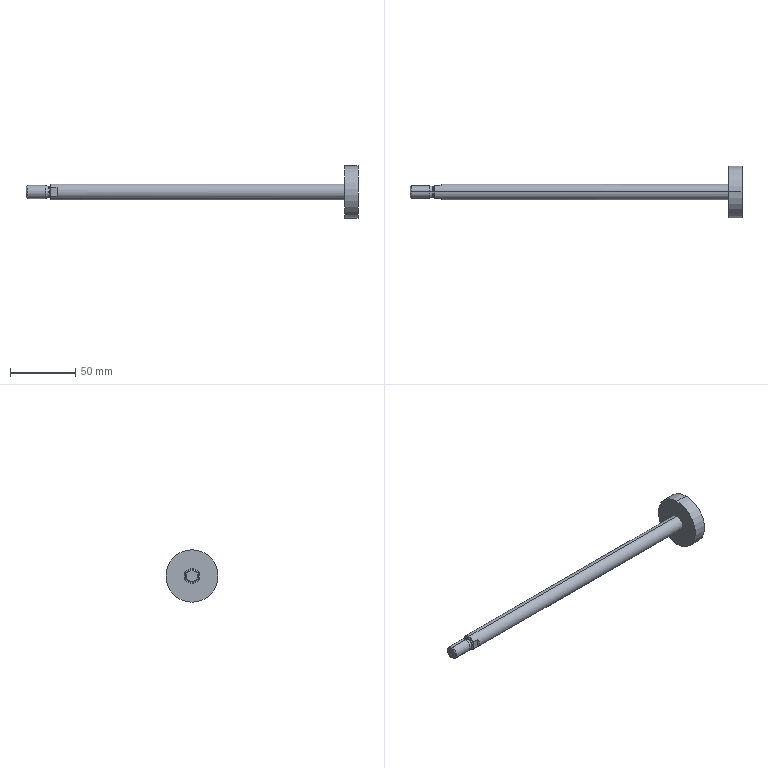Part | SolidWorks | features ICE 6, Draft 2, Chamfer 1, Fillet 1, Revolution 1 | 1 solid | 24 faces | box 253.7 x 40 x 40 mm | volume 39349 mm3 | cylinder 8 | plane 8 | torus 4 | cone 4 | commonest cylinder face diameters 8.2 x2 10 x2 12 x2 40 x2
STEP:
#1=CARTESIAN_POINT('',(-7.699,0.,-4.136));
#2=VERTEX_POINT('',#1);
#3=CARTESIAN_POINT('',(-7.699,0.,4.136));
#4=VERTEX_POINT('',#3);
#5=CARTESIAN_POINT('',(-7.699,0.,0.));
#6=DIRECTION('',(-1.,0.,0.));
#7=DIRECTION('',(0.,0.,1.));
#8=AXIS2_PLACEMENT_3D('',#5,#6,#7);
#9=CIRCLE('',#8,4.136);
#10=EDGE_CURVE('',#2,#4,#9,.T.);
#11=ORIENTED_EDGE('',*,*,#10,.F.);
#12=CARTESIAN_POINT('',(-7.494,0.,-4.1));
#13=VERTEX_POINT('',#12);
#14=CARTESIAN_POINT('',(-7.494,0.,-4.7));
#15=DIRECTION('',(0.,1.,0.));
#16=DIRECTION('',(0.,0.,1.));
#17=AXIS2_PLACEMENT_3D('',#14,#15,#16);
#18=CIRCLE('',#17,0.6);
#19=EDGE_CURVE('',#2,#13,#18,.T.);
#20=ORIENTED_EDGE('',*,*,#19,.T.);
#21=CARTESIAN_POINT('',(-7.494,0.,4.1));
#22=VERTEX_POINT('',#21);
#23=CARTESIAN_POINT('',(-7.494,0.,0.));
#24=DIRECTION('',(1.,0.,0.));
#25=DIRECTION('',(0.,0.,1.));
#26=AXIS2_PLACEMENT_3D('',#23,#24,#25);
#27=CIRCLE('',#26,4.1);
#28=EDGE_CURVE('',#22,#13,#27,.T.);
#29=ORIENTED_EDGE('',*,*,#28,.F.);
#30=CARTESIAN_POINT('',(-7.494,0.,4.7));
#31=DIRECTION('',(0.,-1.,0.));
#32=DIRECTION('',(0.,0.,-1.));
#33=AXIS2_PLACEMENT_3D('',#30,#31,#32);
#34=CIRCLE('',#33,0.6);
#35=EDGE_CURVE('',#4,#22,#34,.T.);
#36=ORIENTED_EDGE('',*,*,#35,.F.);
#37=EDGE_LOOP('',(#11,#20,#29,#36));
#38=FACE_OUTER_BOUND('',#37,.T.);
#39=CARTESIAN_POINT('',(-7.494,0.,0.));
#40=DIRECTION('',(-1.,0.,0.));
#41=DIRECTION('',(0.,0.,1.));
#42=AXIS2_PLACEMENT_3D('',#39,#40,#41);
#43=TOROIDAL_SURFACE('',#42,4.7,0.6);
#44=ADVANCED_FACE('',(#38),#43,.F.);
#45=CARTESIAN_POINT('',(-6.7,0.,-4.1));
#46=VERTEX_POINT('',#45);
#47=CARTESIAN_POINT('',(-6.7,0.,4.1));
#48=VERTEX_POINT('',#47);
#49=CARTESIAN_POINT('',(-6.7,0.,0.));
#50=DIRECTION('',(-1.,0.,0.));
#51=DIRECTION('',(0.,0.,1.));
#52=AXIS2_PLACEMENT_3D('',#49,#50,#51);
#53=CIRCLE('',#52,4.1);
#54=EDGE_CURVE('',#46,#48,#53,.T.);
#55=ORIENTED_EDGE('',*,*,#54,.F.);
#56=CARTESIAN_POINT('',(-6.1,0.,-4.7));
#57=VERTEX_POINT('',#56);
#58=CARTESIAN_POINT('',(-6.7,0.,-4.7));
#59=DIRECTION('',(0.,1.,0.));
#60=DIRECTION('',(0.,0.,1.));
#61=AXIS2_PLACEMENT_3D('',#58,#59,#60);
#62=CIRCLE('',#61,0.6);
#63=EDGE_CURVE('',#46,#57,#62,.T.);
#64=ORIENTED_EDGE('',*,*,#63,.T.);
#65=CARTESIAN_POINT('',(-6.1,0.,4.7));
#66=VERTEX_POINT('',#65);
#67=CARTESIAN_POINT('',(-6.1,0.,0.));
#68=DIRECTION('',(1.,0.,0.));
#69=DIRECTION('',(0.,0.,1.));
#70=AXIS2_PLACEMENT_3D('',#67,#68,#69);
#71=CIRCLE('',#70,4.7);
#72=EDGE_CURVE('',#66,#57,#71,.T.);
#73=ORIENTED_EDGE('',*,*,#72,.F.);
#74=CARTESIAN_POINT('',(-6.7,0.,4.7));
#75=DIRECTION('',(0.,-1.,0.));
#76=DIRECTION('',(0.,0.,-1.));
#77=AXIS2_PLACEMENT_3D('',#74,#75,#76);
#78=CIRCLE('',#77,0.6);
#79=EDGE_CURVE('',#48,#66,#78,.T.);
#80=ORIENTED_EDGE('',*,*,#79,.F.);
#81=EDGE_LOOP('',(#55,#64,#73,#80));
#82=FACE_OUTER_BOUND('',#81,.T.);
#83=CARTESIAN_POINT('',(-6.7,0.,0.));
#84=DIRECTION('',(-1.,0.,0.));
#85=DIRECTION('',(0.,0.,1.));
#86=AXIS2_PLACEMENT_3D('',#83,#84,#85);
#87=TOROIDAL_SURFACE('',#86,4.7,0.6);
#88=ADVANCED_FACE('',(#82),#87,.F.);
#89=CARTESIAN_POINT('',(-25.1,0.,4.233));
#90=VERTEX_POINT('',#89);
#91=CARTESIAN_POINT('',(-25.1,0.,-4.233));
#92=VERTEX_POINT('',#91);
#93=CARTESIAN_POINT('',(-25.1,0.,0.));
#94=DIRECTION('',(-1.,0.,0.));
#95=DIRECTION('',(0.,0.,1.));
#96=AXIS2_PLACEMENT_3D('',#93,#94,#95);
#97=CIRCLE('',#96,4.233);
#98=EDGE_CURVE('',#90,#92,#97,.T.);
#99=ORIENTED_EDGE('',*,*,#98,.F.);
#100=CARTESIAN_POINT('',(-24.333,0.,5.));
#101=VERTEX_POINT('',#100);
#102=CARTESIAN_POINT('',(-25.1,0.,4.233));
#103=DIRECTION('',(0.7071,0.,0.7071));
#104=VECTOR('',#103,1000.);
#105=LINE('',#102,#104);
#106=EDGE_CURVE('',#90,#101,#105,.T.);
#107=ORIENTED_EDGE('',*,*,#106,.T.);
#108=CARTESIAN_POINT('',(-24.333,0.,-5.));
#109=VERTEX_POINT('',#108);
#110=CARTESIAN_POINT('',(-24.333,0.,0.));
#111=DIRECTION('',(1.,0.,0.));
#112=DIRECTION('',(0.,0.,1.));
#113=AXIS2_PLACEMENT_3D('',#110,#111,#112);
#114=CIRCLE('',#113,5.);
#115=EDGE_CURVE('',#109,#101,#114,.T.);
#116=ORIENTED_EDGE('',*,*,#115,.F.);
#117=CARTESIAN_POINT('',(-25.1,0.,-4.233));
#118=DIRECTION('',(0.7071,0.,-0.7071));
#119=VECTOR('',#118,1000.);
#120=LINE('',#117,#119);
#121=EDGE_CURVE('',#92,#109,#120,.T.);
#122=ORIENTED_EDGE('',*,*,#121,.F.);
#123=EDGE_LOOP('',(#99,#107,#116,#122));
#124=FACE_OUTER_BOUND('',#123,.T.);
#125=CARTESIAN_POINT('',(-25.1,0.,0.));
#126=DIRECTION('',(1.,0.,0.));
#127=DIRECTION('',(0.,0.,-1.));
#128=AXIS2_PLACEMENT_3D('',#125,#126,#127);
#129=CONICAL_SURFACE('',#128,4.233,0.7854);
#130=ADVANCED_FACE('',(#124),#129,.T.);
#131=ORIENTED_EDGE('',*,*,#115,.T.);
#132=CARTESIAN_POINT('',(-10.073,0.,5.));
#133=VERTEX_POINT('',#132);
#134=CARTESIAN_POINT('',(-25.1,0.,5.));
#135=DIRECTION('',(1.,0.,0.));
#136=VECTOR('',#135,1000.);
#137=LINE('',#134,#136);
#138=EDGE_CURVE('',#101,#133,#137,.T.);
#139=ORIENTED_EDGE('',*,*,#138,.T.);
#140=CARTESIAN_POINT('',(-10.073,0.,-5.));
#141=VERTEX_POINT('',#140);
#142=CARTESIAN_POINT('',(-10.073,0.,0.));
#143=DIRECTION('',(-1.,0.,0.));
#144=DIRECTION('',(0.,0.,1.));
#145=AXIS2_PLACEMENT_3D('',#142,#143,#144);
#146=CIRCLE('',#145,5.);
#147=EDGE_CURVE('',#133,#141,#146,.T.);
#148=ORIENTED_EDGE('',*,*,#147,.T.);
#149=CARTESIAN_POINT('',(-25.1,0.,-5.));
#150=DIRECTION('',(1.,0.,0.));
#151=VECTOR('',#150,1000.);
#152=LINE('',#149,#151);
#153=EDGE_CURVE('',#109,#141,#152,.T.);
#154=ORIENTED_EDGE('',*,*,#153,.F.);
#155=EDGE_LOOP('',(#131,#139,#148,#154));
#156=FACE_OUTER_BOUND('',#155,.T.);
#157=CARTESIAN_POINT('',(-25.1,0.,0.));
#158=DIRECTION('',(1.,0.,0.));
#159=DIRECTION('',(0.,0.,-1.));
#160=AXIS2_PLACEMENT_3D('',#157,#158,#159);
#161=CYLINDRICAL_SURFACE('',#160,5.);
#162=ADVANCED_FACE('',(#156),#161,.T.);
#163=CARTESIAN_POINT('',(-7.699,0.,0.));
#164=DIRECTION('',(-1.,0.,0.));
#165=DIRECTION('',(0.,0.,1.));
#166=AXIS2_PLACEMENT_3D('',#163,#164,#165);
#167=CIRCLE('',#166,4.136);
#168=EDGE_CURVE('',#4,#2,#167,.T.);
#169=ORIENTED_EDGE('',*,*,#168,.T.);
#170=CARTESIAN_POINT('',(-7.6,0.,-4.1));
#171=DIRECTION('',(-0.9397,0.,-0.342));
#172=VECTOR('',#171,1000.);
#173=LINE('',#170,#172);
#174=EDGE_CURVE('',#2,#141,#173,.T.);
#175=ORIENTED_EDGE('',*,*,#174,.T.);
#176=ORIENTED_EDGE('',*,*,#147,.F.);
#177=CARTESIAN_POINT('',(-7.6,0.,4.1));
#178=DIRECTION('',(-0.9397,0.,0.342));
#179=VECTOR('',#178,1000.);
#180=LINE('',#177,#179);
#181=EDGE_CURVE('',#4,#133,#180,.T.);
#182=ORIENTED_EDGE('',*,*,#181,.F.);
#183=EDGE_LOOP('',(#169,#175,#176,#182));
#184=FACE_OUTER_BOUND('',#183,.T.);
#185=CARTESIAN_POINT('',(-7.6,0.,0.));
#186=DIRECTION('',(-1.,0.,0.));
#187=DIRECTION('',(0.,0.,1.));
#188=AXIS2_PLACEMENT_3D('',#185,#186,#187);
#189=CONICAL_SURFACE('',#188,4.1,0.3491);
#190=ADVANCED_FACE('',(#184),#189,.T.);
#191=CARTESIAN_POINT('',(-7.494,0.,0.));
#192=DIRECTION('',(1.,0.,0.));
#193=DIRECTION('',(0.,0.,1.));
#194=AXIS2_PLACEMENT_3D('',#191,#192,#193);
#195=CIRCLE('',#194,4.1);
#196=EDGE_CURVE('',#13,#22,#195,.T.);
#197=ORIENTED_EDGE('',*,*,#196,.T.);
#198=CARTESIAN_POINT('',(-7.6,0.,4.1));
#199=DIRECTION('',(1.,0.,0.));
#200=VECTOR('',#199,1000.);
#201=LINE('',#198,#200);
#202=EDGE_CURVE('',#22,#48,#201,.T.);
#203=ORIENTED_EDGE('',*,*,#202,.T.);
#204=CARTESIAN_POINT('',(-6.7,0.,0.));
#205=DIRECTION('',(-1.,0.,0.));
#206=DIRECTION('',(0.,0.,1.));
#207=AXIS2_PLACEMENT_3D('',#204,#205,#206);
#208=CIRCLE('',#207,4.1);
#209=EDGE_CURVE('',#48,#46,#208,.T.);
#210=ORIENTED_EDGE('',*,*,#209,.T.);
#211=CARTESIAN_POINT('',(-7.6,0.,-4.1));
#212=DIRECTION('',(1.,0.,0.));
#213=VECTOR('',#212,1000.);
#214=LINE('',#211,#213);
#215=EDGE_CURVE('',#13,#46,#214,.T.);
#216=ORIENTED_EDGE('',*,*,#215,.F.);
#217=EDGE_LOOP('',(#197,#203,#210,#216));
#218=FACE_OUTER_BOUND('',#217,.T.);
#219=CARTESIAN_POINT('',(-7.6,0.,0.));
#220=DIRECTION('',(1.,0.,0.));
#221=DIRECTION('',(0.,0.,-1.));
#222=AXIS2_PLACEMENT_3D('',#219,#220,#221);
#223=CYLINDRICAL_SURFACE('',#222,4.1);
#224=ADVANCED_FACE('',(#218),#223,.T.);
#225=CARTESIAN_POINT('',(-6.1,0.,6.));
#226=VERTEX_POINT('',#225);
#227=CARTESIAN_POINT('',(-6.1,5.,3.317));
#228=VERTEX_POINT('',#227);
#229=CARTESIAN_POINT('',(-6.1,0.,0.));
#230=DIRECTION('',(-1.,0.,0.));
#231=DIRECTION('',(0.,0.,1.));
#232=AXIS2_PLACEMENT_3D('',#229,#230,#231);
#233=CIRCLE('',#232,6.);
#234=EDGE_CURVE('',#226,#228,#233,.T.);
#235=ORIENTED_EDGE('',*,*,#234,.F.);
#236=CARTESIAN_POINT('',(218.6,0.,6.));
#237=VERTEX_POINT('',#236);
#238=CARTESIAN_POINT('',(-6.1,0.,6.));
#239=DIRECTION('',(1.,0.,0.));
#240=VECTOR('',#239,1000.);
#241=LINE('',#238,#240);
#242=EDGE_CURVE('',#226,#237,#241,.T.);
#243=ORIENTED_EDGE('',*,*,#242,.T.);
#244=CARTESIAN_POINT('',(218.6,0.,-6.));
#245=VERTEX_POINT('',#244);
#246=CARTESIAN_POINT('',(218.6,0.,0.));
#247=DIRECTION('',(-1.,0.,0.));
#248=DIRECTION('',(0.,0.,1.));
#249=AXIS2_PLACEMENT_3D('',#246,#247,#248);
#250=CIRCLE('',#249,6.);
#251=EDGE_CURVE('',#237,#245,#250,.T.);
#252=ORIENTED_EDGE('',*,*,#251,.T.);
#253=CARTESIAN_POINT('',(-6.1,0.,-6.));
#254=VERTEX_POINT('',#253);
#255=CARTESIAN_POINT('',(-6.1,0.,-6.));
#256=DIRECTION('',(1.,0.,0.));
#257=VECTOR('',#256,1000.);
#258=LINE('',#255,#257);
#259=EDGE_CURVE('',#254,#245,#258,.T.);
#260=ORIENTED_EDGE('',*,*,#259,.F.);
#261=CARTESIAN_POINT('',(-6.1,5.,-3.317));
#262=VERTEX_POINT('',#261);
#263=CARTESIAN_POINT('',(-6.1,0.,0.));
#264=DIRECTION('',(-1.,0.,0.));
#265=DIRECTION('',(0.,0.,1.));
#266=AXIS2_PLACEMENT_3D('',#263,#264,#265);
#267=CIRCLE('',#266,6.);
#268=EDGE_CURVE('',#262,#254,#267,.T.);
#269=ORIENTED_EDGE('',*,*,#268,.F.);
#270=CARTESIAN_POINT('',(-1.4,5.,-3.317));
#271=VERTEX_POINT('',#270);
#272=CARTESIAN_POINT('',(-1.4,5.,-3.317));
#273=DIRECTION('',(-1.,0.,0.));
#274=VECTOR('',#273,1000.);
#275=LINE('',#272,#274);
#276=EDGE_CURVE('',#271,#262,#275,.T.);
#277=ORIENTED_EDGE('',*,*,#276,.F.);
#278=CARTESIAN_POINT('',(-1.4,5.,3.317));
#279=VERTEX_POINT('',#278);
#280=CARTESIAN_POINT('',(-1.4,5.,3.317));
#281=CARTESIAN_POINT('',(-0.6061,6.375,1.244));
#282=CARTESIAN_POINT('',(-0.6061,6.375,-1.244));
#283=CARTESIAN_POINT('',(-1.4,5.,-3.317));
#284=(BOUNDED_CURVE()B_SPLINE_CURVE(3,(#280,#281,#282,#283),.UNSPECIFIED.,.F.,.F.)B_SPLINE_CURVE_WITH_KNOTS((4,4),(5.697,6.869),.UNSPECIFIED.)CURVE()GEOMETRIC_REPRESENTATION_ITEM()RATIONAL_B_SPLINE_CURVE((1.,0.8889,0.8889,1.))REPRESENTATION_ITEM(''));
#285=EDGE_CURVE('',#279,#271,#284,.T.);
#286=ORIENTED_EDGE('',*,*,#285,.F.);
#287=CARTESIAN_POINT('',(-1.4,5.,3.317));
#288=DIRECTION('',(-1.,0.,0.));
#289=VECTOR('',#288,1000.);
#290=LINE('',#287,#289);
#291=EDGE_CURVE('',#279,#228,#290,.T.);
#292=ORIENTED_EDGE('',*,*,#291,.T.);
#293=EDGE_LOOP('',(#235,#243,#252,#260,#269,#277,#286,#292));
#294=FACE_OUTER_BOUND('',#293,.T.);
#295=CARTESIAN_POINT('',(-6.1,0.,0.));
#296=DIRECTION('',(1.,0.,0.));
#297=DIRECTION('',(0.,0.,-1.));
#298=AXIS2_PLACEMENT_3D('',#295,#296,#297);
#299=CYLINDRICAL_SURFACE('',#298,6.);
#300=ADVANCED_FACE('',(#294),#299,.T.);
#301=CARTESIAN_POINT('',(228.6,0.,20.));
#302=VERTEX_POINT('',#301);
#303=CARTESIAN_POINT('',(228.6,0.,-20.));
#304=VERTEX_POINT('',#303);
#305=CARTESIAN_POINT('',(228.6,0.,0.));
#306=DIRECTION('',(-1.,0.,0.));
#307=DIRECTION('',(0.,0.,1.));
#308=AXIS2_PLACEMENT_3D('',#305,#306,#307);
#309=CIRCLE('',#308,20.);
#310=EDGE_CURVE('',#302,#304,#309,.T.);
#311=ORIENTED_EDGE('',*,*,#310,.T.);
#312=CARTESIAN_POINT('',(218.6,0.,-20.));
#313=VERTEX_POINT('',#312);
#314=CARTESIAN_POINT('',(228.6,0.,-20.));
#315=DIRECTION('',(-1.,0.,0.));
#316=VECTOR('',#315,1000.);
#317=LINE('',#314,#316);
#318=EDGE_CURVE('',#304,#313,#317,.T.);
#319=ORIENTED_EDGE('',*,*,#318,.T.);
#320=CARTESIAN_POINT('',(218.6,0.,20.));
#321=VERTEX_POINT('',#320);
#322=CARTESIAN_POINT('',(218.6,0.,0.));
#323=DIRECTION('',(-1.,0.,0.));
#324=DIRECTION('',(0.,0.,1.));
#325=AXIS2_PLACEMENT_3D('',#322,#323,#324);
#326=CIRCLE('',#325,20.);
#327=EDGE_CURVE('',#321,#313,#326,.T.);
#328=ORIENTED_EDGE('',*,*,#327,.F.);
#329=CARTESIAN_POINT('',(228.6,0.,20.));
#330=DIRECTION('',(-1.,0.,0.));
#331=VECTOR('',#330,1000.);
#332=LINE('',#329,#331);
#333=EDGE_CURVE('',#302,#321,#332,.T.);
#334=ORIENTED_EDGE('',*,*,#333,.F.);
#335=EDGE_LOOP('',(#311,#319,#328,#334));
#336=FACE_OUTER_BOUND('',#335,.T.);
#337=CARTESIAN_POINT('',(228.6,0.,0.));
#338=DIRECTION('',(-1.,0.,0.));
#339=DIRECTION('',(0.,0.,1.));
#340=AXIS2_PLACEMENT_3D('',#337,#338,#339);
#341=CYLINDRICAL_SURFACE('',#340,20.);
#342=ADVANCED_FACE('',(#336),#341,.T.);
#343=ORIENTED_EDGE('',*,*,#318,.F.);
#344=CARTESIAN_POINT('',(228.6,0.,0.));
#345=DIRECTION('',(-1.,0.,0.));
#346=DIRECTION('',(0.,0.,1.));
#347=AXIS2_PLACEMENT_3D('',#344,#345,#346);
#348=CIRCLE('',#347,20.);
#349=EDGE_CURVE('',#304,#302,#348,.T.);
#350=ORIENTED_EDGE('',*,*,#349,.T.);
#351=ORIENTED_EDGE('',*,*,#333,.T.);
#352=CARTESIAN_POINT('',(218.6,0.,0.));
#353=DIRECTION('',(-1.,0.,0.));
#354=DIRECTION('',(0.,0.,1.));
#355=AXIS2_PLACEMENT_3D('',#352,#353,#354);
#356=CIRCLE('',#355,20.);
#357=EDGE_CURVE('',#313,#321,#356,.T.);
#358=ORIENTED_EDGE('',*,*,#357,.F.);
#359=EDGE_LOOP('',(#343,#350,#351,#358));
#360=FACE_OUTER_BOUND('',#359,.T.);
#361=CARTESIAN_POINT('',(228.6,0.,0.));
#362=DIRECTION('',(-1.,0.,0.));
#363=DIRECTION('',(0.,0.,1.));
#364=AXIS2_PLACEMENT_3D('',#361,#362,#363);
#365=CYLINDRICAL_SURFACE('',#364,20.);
#366=ADVANCED_FACE('',(#360),#365,.T.);
#367=ORIENTED_EDGE('',*,*,#310,.F.);
#368=ORIENTED_EDGE('',*,*,#349,.F.);
#369=EDGE_LOOP('',(#367,#368));
#370=FACE_OUTER_BOUND('',#369,.T.);
#371=CARTESIAN_POINT('',(228.6,20.,0.));
#372=DIRECTION('',(1.,0.,0.));
#373=DIRECTION('',(0.,0.,-1.));
#374=AXIS2_PLACEMENT_3D('',#371,#372,#373);
#375=PLANE('',#374);
#376=ADVANCED_FACE('',(#370),#375,.T.);
#377=CARTESIAN_POINT('',(218.6,0.,0.));
#378=DIRECTION('',(-1.,0.,0.));
#379=DIRECTION('',(0.,0.,1.));
#380=AXIS2_PLACEMENT_3D('',#377,#378,#379);
#381=CIRCLE('',#380,6.);
#382=EDGE_CURVE('',#245,#237,#381,.T.);
#383=ORIENTED_EDGE('',*,*,#382,.F.);
#384=ORIENTED_EDGE('',*,*,#251,.F.);
#385=EDGE_LOOP('',(#383,#384));
#386=FACE_BOUND('',#385,.T.);
#387=ORIENTED_EDGE('',*,*,#327,.T.);
#388=ORIENTED_EDGE('',*,*,#357,.T.);
#389=EDGE_LOOP('',(#387,#388));
#390=FACE_OUTER_BOUND('',#389,.T.);
#391=CARTESIAN_POINT('',(218.6,0.,0.));
#392=DIRECTION('',(-1.,0.,0.));
#393=DIRECTION('',(0.,0.,1.));
#394=AXIS2_PLACEMENT_3D('',#391,#392,#393);
#395=PLANE('',#394);
#396=ADVANCED_FACE('',(#386,#390),#395,.T.);
#397=ORIENTED_EDGE('',*,*,#242,.F.);
#398=CARTESIAN_POINT('',(-6.1,-5.,3.317));
#399=VERTEX_POINT('',#398);
#400=CARTESIAN_POINT('',(-6.1,0.,0.));
#401=DIRECTION('',(-1.,0.,0.));
#402=DIRECTION('',(0.,0.,1.));
#403=AXIS2_PLACEMENT_3D('',#400,#401,#402);
#404=CIRCLE('',#403,6.);
#405=EDGE_CURVE('',#399,#226,#404,.T.);
#406=ORIENTED_EDGE('',*,*,#405,.F.);
#407=CARTESIAN_POINT('',(-1.4,-5.,3.317));
#408=VERTEX_POINT('',#407);
#409=CARTESIAN_POINT('',(-1.4,-5.,3.317));
#410=DIRECTION('',(-1.,0.,0.));
#411=VECTOR('',#410,1000.);
#412=LINE('',#409,#411);
#413=EDGE_CURVE('',#408,#399,#412,.T.);
#414=ORIENTED_EDGE('',*,*,#413,.F.);
#415=CARTESIAN_POINT('',(-1.4,-5.,-3.317));
#416=VERTEX_POINT('',#415);
#417=CARTESIAN_POINT('',(-1.4,-5.,-3.317));
#418=CARTESIAN_POINT('',(-0.6061,-6.375,-1.244));
#419=CARTESIAN_POINT('',(-0.6061,-6.375,1.244));
#420=CARTESIAN_POINT('',(-1.4,-5.,3.317));
#421=(BOUNDED_CURVE()B_SPLINE_CURVE(3,(#417,#418,#419,#420),.UNSPECIFIED.,.F.,.F.)B_SPLINE_CURVE_WITH_KNOTS((4,4),(5.697,6.869),.UNSPECIFIED.)CURVE()GEOMETRIC_REPRESENTATION_ITEM()RATIONAL_B_SPLINE_CURVE((1.,0.8889,0.8889,1.))REPRESENTATION_ITEM(''));
#422=EDGE_CURVE('',#416,#408,#421,.T.);
#423=ORIENTED_EDGE('',*,*,#422,.F.);
#424=CARTESIAN_POINT('',(-6.1,-5.,-3.317));
#425=VERTEX_POINT('',#424);
#426=CARTESIAN_POINT('',(-1.4,-5.,-3.317));
#427=DIRECTION('',(-1.,0.,0.));
#428=VECTOR('',#427,1000.);
#429=LINE('',#426,#428);
#430=EDGE_CURVE('',#416,#425,#429,.T.);
#431=ORIENTED_EDGE('',*,*,#430,.T.);
#432=CARTESIAN_POINT('',(-6.1,0.,0.));
#433=DIRECTION('',(-1.,0.,0.));
#434=DIRECTION('',(0.,0.,1.));
#435=AXIS2_PLACEMENT_3D('',#432,#433,#434);
#436=CIRCLE('',#435,6.);
#437=EDGE_CURVE('',#254,#425,#436,.T.);
#438=ORIENTED_EDGE('',*,*,#437,.F.);
#439=ORIENTED_EDGE('',*,*,#259,.T.);
#440=ORIENTED_EDGE('',*,*,#382,.T.);
#441=EDGE_LOOP('',(#397,#406,#414,#423,#431,#438,#439,#440));
#442=FACE_OUTER_BOUND('',#441,.T.);
#443=CARTESIAN_POINT('',(-6.1,0.,0.));
#444=DIRECTION('',(1.,0.,0.));
#445=DIRECTION('',(0.,0.,-1.));
#446=AXIS2_PLACEMENT_3D('',#443,#444,#445);
#447=CYLINDRICAL_SURFACE('',#446,6.);
#448=ADVANCED_FACE('',(#442),#447,.T.);
#449=ORIENTED_EDGE('',*,*,#72,.T.);
#450=CARTESIAN_POINT('',(-6.1,0.,0.));
#451=DIRECTION('',(1.,0.,0.));
#452=DIRECTION('',(0.,0.,1.));
#453=AXIS2_PLACEMENT_3D('',#450,#451,#452);
#454=CIRCLE('',#453,4.7);
#455=EDGE_CURVE('',#57,#66,#454,.T.);
#456=ORIENTED_EDGE('',*,*,#455,.T.);
#457=EDGE_LOOP('',(#449,#456));
#458=FACE_BOUND('',#457,.T.);
#459=CARTESIAN_POINT('',(-6.1,-5.,3.317));
#460=DIRECTION('',(0.,0.,-1.));
#461=VECTOR('',#460,1000.);
#462=LINE('',#459,#461);
#463=EDGE_CURVE('',#399,#425,#462,.T.);
#464=ORIENTED_EDGE('',*,*,#463,.F.);
#465=ORIENTED_EDGE('',*,*,#405,.T.);
#466=ORIENTED_EDGE('',*,*,#234,.T.);
#467=CARTESIAN_POINT('',(-6.1,5.,-3.317));
#468=DIRECTION('',(0.,0.,1.));
#469=VECTOR('',#468,1000.);
#470=LINE('',#467,#469);
#471=EDGE_CURVE('',#262,#228,#470,.T.);
#472=ORIENTED_EDGE('',*,*,#471,.F.);
#473=ORIENTED_EDGE('',*,*,#268,.T.);
#474=ORIENTED_EDGE('',*,*,#437,.T.);
#475=EDGE_LOOP('',(#464,#465,#466,#472,#473,#474));
#476=FACE_OUTER_BOUND('',#475,.T.);
#477=CARTESIAN_POINT('',(-6.1,0.,0.));
#478=DIRECTION('',(-1.,0.,0.));
#479=DIRECTION('',(0.,0.,1.));
#480=AXIS2_PLACEMENT_3D('',#477,#478,#479);
#481=PLANE('',#480);
#482=ADVANCED_FACE('',(#458,#476),#481,.T.);
#483=ORIENTED_EDGE('',*,*,#471,.T.);
#484=ORIENTED_EDGE('',*,*,#291,.F.);
#485=CARTESIAN_POINT('',(-1.4,5.,-3.317));
#486=DIRECTION('',(0.,0.,1.));
#487=VECTOR('',#486,1000.);
#488=LINE('',#485,#487);
#489=EDGE_CURVE('',#271,#279,#488,.T.);
#490=ORIENTED_EDGE('',*,*,#489,.F.);
#491=ORIENTED_EDGE('',*,*,#276,.T.);
#492=EDGE_LOOP('',(#483,#484,#490,#491));
#493=FACE_OUTER_BOUND('',#492,.T.);
#494=CARTESIAN_POINT('',(-1.4,5.,-3.317));
#495=DIRECTION('',(0.,-1.,0.));
#496=DIRECTION('',(0.,0.,-1.));
#497=AXIS2_PLACEMENT_3D('',#494,#495,#496);
#498=PLANE('',#497);
#499=ADVANCED_FACE('',(#493),#498,.F.);
#500=ORIENTED_EDGE('',*,*,#285,.T.);
#501=ORIENTED_EDGE('',*,*,#489,.T.);
#502=EDGE_LOOP('',(#500,#501));
#503=FACE_OUTER_BOUND('',#502,.T.);
#504=CARTESIAN_POINT('',(-1.4,5.,-3.317));
#505=DIRECTION('',(-0.866,0.5,0.));
#506=DIRECTION('',(-0.5,-0.866,0.));
#507=AXIS2_PLACEMENT_3D('',#504,#505,#506);
#508=PLANE('',#507);
#509=ADVANCED_FACE('',(#503),#508,.T.);
#510=ORIENTED_EDGE('',*,*,#463,.T.);
#511=ORIENTED_EDGE('',*,*,#430,.F.);
#512=CARTESIAN_POINT('',(-1.4,-5.,3.317));
#513=DIRECTION('',(0.,0.,-1.));
#514=VECTOR('',#513,1000.);
#515=LINE('',#512,#514);
#516=EDGE_CURVE('',#408,#416,#515,.T.);
#517=ORIENTED_EDGE('',*,*,#516,.F.);
#518=ORIENTED_EDGE('',*,*,#413,.T.);
#519=EDGE_LOOP('',(#510,#511,#517,#518));
#520=FACE_OUTER_BOUND('',#519,.T.);
#521=CARTESIAN_POINT('',(-1.4,-5.,3.317));
#522=DIRECTION('',(0.,1.,0.));
#523=DIRECTION('',(0.,0.,1.));
#524=AXIS2_PLACEMENT_3D('',#521,#522,#523);
#525=PLANE('',#524);
#526=ADVANCED_FACE('',(#520),#525,.F.);
#527=ORIENTED_EDGE('',*,*,#422,.T.);
#528=ORIENTED_EDGE('',*,*,#516,.T.);
#529=EDGE_LOOP('',(#527,#528));
#530=FACE_OUTER_BOUND('',#529,.T.);
#531=CARTESIAN_POINT('',(-1.4,-5.,3.317));
#532=DIRECTION('',(-0.866,-0.5,0.));
#533=DIRECTION('',(0.5,-0.866,0.));
#534=AXIS2_PLACEMENT_3D('',#531,#532,#533);
#535=PLANE('',#534);
#536=ADVANCED_FACE('',(#530),#535,.T.);
#537=ORIENTED_EDGE('',*,*,#202,.F.);
#538=ORIENTED_EDGE('',*,*,#28,.T.);
#539=ORIENTED_EDGE('',*,*,#215,.T.);
#540=ORIENTED_EDGE('',*,*,#54,.T.);
#541=EDGE_LOOP('',(#537,#538,#539,#540));
#542=FACE_OUTER_BOUND('',#541,.T.);
#543=CARTESIAN_POINT('',(-7.6,0.,0.));
#544=DIRECTION('',(1.,0.,0.));
#545=DIRECTION('',(0.,0.,-1.));
#546=AXIS2_PLACEMENT_3D('',#543,#544,#545);
#547=CYLINDRICAL_SURFACE('',#546,4.1);
#548=ADVANCED_FACE('',(#542),#547,.T.);
#549=ORIENTED_EDGE('',*,*,#174,.F.);
#550=ORIENTED_EDGE('',*,*,#10,.T.);
#551=ORIENTED_EDGE('',*,*,#181,.T.);
#552=CARTESIAN_POINT('',(-10.073,0.,0.));
#553=DIRECTION('',(-1.,0.,0.));
#554=DIRECTION('',(0.,0.,1.));
#555=AXIS2_PLACEMENT_3D('',#552,#553,#554);
#556=CIRCLE('',#555,5.);
#557=EDGE_CURVE('',#141,#133,#556,.T.);
#558=ORIENTED_EDGE('',*,*,#557,.F.);
#559=EDGE_LOOP('',(#549,#550,#551,#558));
#560=FACE_OUTER_BOUND('',#559,.T.);
#561=CARTESIAN_POINT('',(-7.6,0.,0.));
#562=DIRECTION('',(-1.,0.,0.));
#563=DIRECTION('',(0.,0.,1.));
#564=AXIS2_PLACEMENT_3D('',#561,#562,#563);
#565=CONICAL_SURFACE('',#564,4.1,0.3491);
#566=ADVANCED_FACE('',(#560),#565,.T.);
#567=ORIENTED_EDGE('',*,*,#138,.F.);
#568=CARTESIAN_POINT('',(-24.333,0.,0.));
#569=DIRECTION('',(1.,0.,0.));
#570=DIRECTION('',(0.,0.,1.));
#571=AXIS2_PLACEMENT_3D('',#568,#569,#570);
#572=CIRCLE('',#571,5.);
#573=EDGE_CURVE('',#101,#109,#572,.T.);
#574=ORIENTED_EDGE('',*,*,#573,.T.);
#575=ORIENTED_EDGE('',*,*,#153,.T.);
#576=ORIENTED_EDGE('',*,*,#557,.T.);
#577=EDGE_LOOP('',(#567,#574,#575,#576));
#578=FACE_OUTER_BOUND('',#577,.T.);
#579=CARTESIAN_POINT('',(-25.1,0.,0.));
#580=DIRECTION('',(1.,0.,0.));
#581=DIRECTION('',(0.,0.,-1.));
#582=AXIS2_PLACEMENT_3D('',#579,#580,#581);
#583=CYLINDRICAL_SURFACE('',#582,5.);
#584=ADVANCED_FACE('',(#578),#583,.T.);
#585=CARTESIAN_POINT('',(-25.1,0.,0.));
#586=DIRECTION('',(-1.,0.,0.));
#587=DIRECTION('',(0.,0.,1.));
#588=AXIS2_PLACEMENT_3D('',#585,#586,#587);
#589=CIRCLE('',#588,4.233);
#590=EDGE_CURVE('',#92,#90,#589,.T.);
#591=ORIENTED_EDGE('',*,*,#590,.T.);
#592=ORIENTED_EDGE('',*,*,#98,.T.);
#593=EDGE_LOOP('',(#591,#592));
#594=FACE_OUTER_BOUND('',#593,.T.);
#595=CARTESIAN_POINT('',(-25.1,0.,0.));
#596=DIRECTION('',(-1.,0.,0.));
#597=DIRECTION('',(0.,0.,1.));
#598=AXIS2_PLACEMENT_3D('',#595,#596,#597);
#599=PLANE('',#598);
#600=ADVANCED_FACE('',(#594),#599,.T.);
#601=ORIENTED_EDGE('',*,*,#106,.F.);
#602=ORIENTED_EDGE('',*,*,#590,.F.);
#603=ORIENTED_EDGE('',*,*,#121,.T.);
#604=ORIENTED_EDGE('',*,*,#573,.F.);
#605=EDGE_LOOP('',(#601,#602,#603,#604));
#606=FACE_OUTER_BOUND('',#605,.T.);
#607=CARTESIAN_POINT('',(-25.1,0.,0.));
#608=DIRECTION('',(1.,0.,0.));
#609=DIRECTION('',(0.,0.,-1.));
#610=AXIS2_PLACEMENT_3D('',#607,#608,#609);
#611=CONICAL_SURFACE('',#610,4.233,0.7854);
#612=ADVANCED_FACE('',(#606),#611,.T.);
#613=ORIENTED_EDGE('',*,*,#63,.F.);
#614=ORIENTED_EDGE('',*,*,#209,.F.);
#615=ORIENTED_EDGE('',*,*,#79,.T.);
#616=ORIENTED_EDGE('',*,*,#455,.F.);
#617=EDGE_LOOP('',(#613,#614,#615,#616));
#618=FACE_OUTER_BOUND('',#617,.T.);
#619=CARTESIAN_POINT('',(-6.7,0.,0.));
#620=DIRECTION('',(-1.,0.,0.));
#621=DIRECTION('',(0.,0.,1.));
#622=AXIS2_PLACEMENT_3D('',#619,#620,#621);
#623=TOROIDAL_SURFACE('',#622,4.7,0.6);
#624=ADVANCED_FACE('',(#618),#623,.F.);
#625=ORIENTED_EDGE('',*,*,#19,.F.);
#626=ORIENTED_EDGE('',*,*,#168,.F.);
#627=ORIENTED_EDGE('',*,*,#35,.T.);
#628=ORIENTED_EDGE('',*,*,#196,.F.);
#629=EDGE_LOOP('',(#625,#626,#627,#628));
#630=FACE_OUTER_BOUND('',#629,.T.);
#631=CARTESIAN_POINT('',(-7.494,0.,0.));
#632=DIRECTION('',(-1.,0.,0.));
#633=DIRECTION('',(0.,0.,1.));
#634=AXIS2_PLACEMENT_3D('',#631,#632,#633);
#635=TOROIDAL_SURFACE('',#634,4.7,0.6);
#636=ADVANCED_FACE('',(#630),#635,.F.);
#637=CLOSED_SHELL('',(#44,#88,#130,#162,#190,#224,#300,#342,#366,#376,#396,#448,#482,#499,#509,#526,#536,#548,#566,#584,#600,#612,#624,#636));
#638=MANIFOLD_SOLID_BREP('',#637);
#639=CARTESIAN_POINT('',(0.,0.,0.));
#640=DIRECTION('',(0.,0.,1.));
#641=DIRECTION('',(1.,0.,0.));
#642=AXIS2_PLACEMENT_3D('',#639,#640,#641);
#643=(LENGTH_UNIT()NAMED_UNIT(*)SI_UNIT(.MILLI.,.METRE.));
#644=UNCERTAINTY_MEASURE_WITH_UNIT(LENGTH_MEASURE(0.00001),#643,'','');
#645=(NAMED_UNIT(*)PLANE_ANGLE_UNIT()SI_UNIT($,.RADIAN.));
#646=(NAMED_UNIT(*)SI_UNIT($,.STERADIAN.)SOLID_ANGLE_UNIT());
#647=(GEOMETRIC_REPRESENTATION_CONTEXT(3)GLOBAL_UNCERTAINTY_ASSIGNED_CONTEXT((#644))GLOBAL_UNIT_ASSIGNED_CONTEXT((#643,#645,#646))REPRESENTATION_CONTEXT('',''));
#648=ADVANCED_BREP_SHAPE_REPRESENTATION('',(#638,#642),#647);